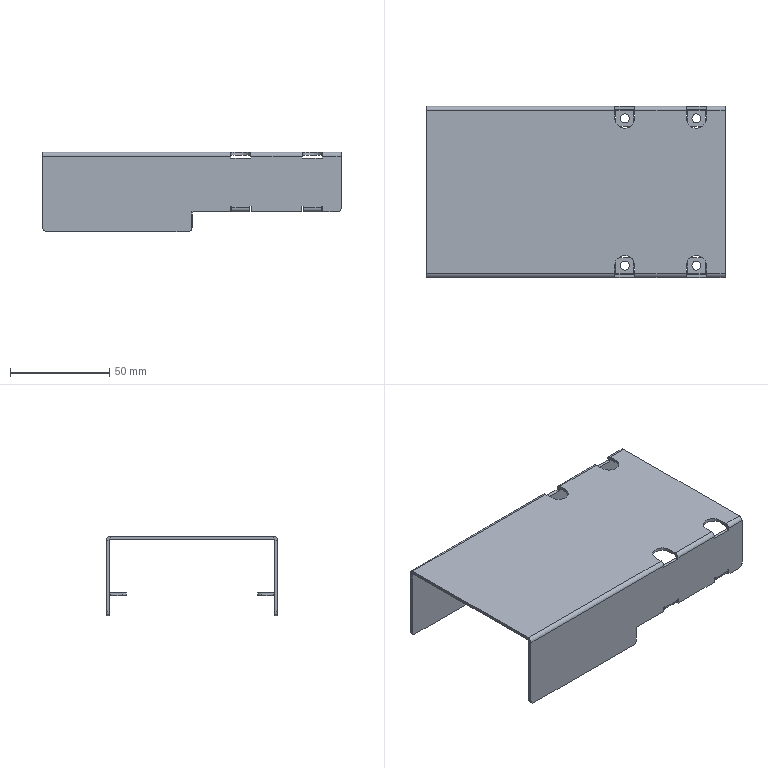Part | STEP file | Belt guard A | 1 solid | 136 faces | box 150 x 86 x 40 mm | volume 33822 mm3 | plane 90 | cylinder 46 | commonest cylinder face diameters 4 x24 1 x10 4.5 x8 10 x4